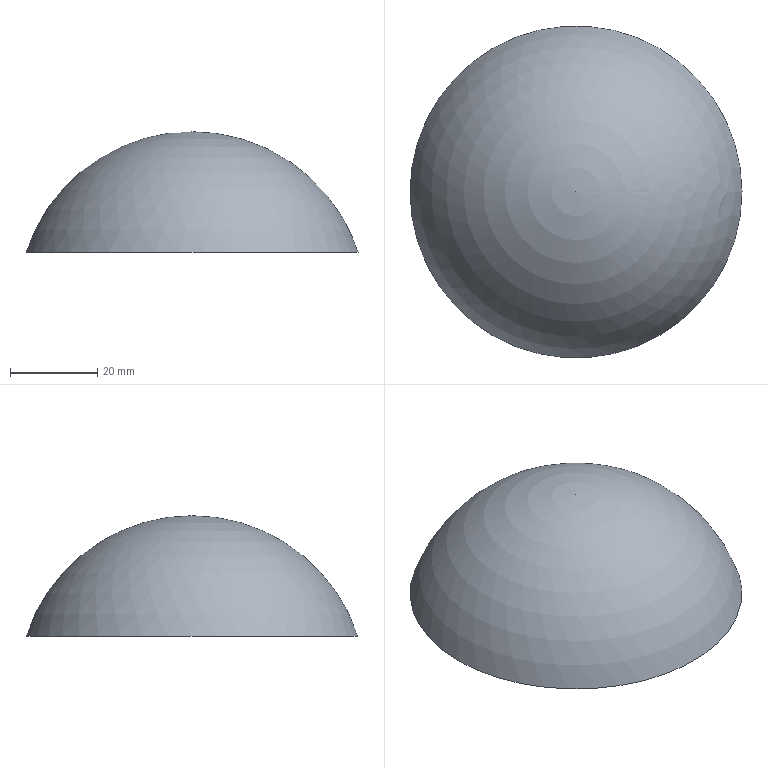Part | STEP file | 21-Guide positioning block | 1 solid | 3 faces | box 76.059 x 76.059 x 27.6 mm | volume 24483 mm3 | sphere 2 | plane 1
STEP:
#1=CARTESIAN_POINT('',(0.,0.,0.));
#2=DIRECTION('',(0.,0.,1.));
#3=DIRECTION('',(1.,0.,0.));
#4=AXIS2_PLACEMENT_3D('',#1,#2,#3);
#5=CARTESIAN_POINT('',(-38.029,0.,12.4));
#6=VERTEX_POINT('',#5);
#7=CARTESIAN_POINT('',(38.029,0.,12.4));
#8=VERTEX_POINT('',#7);
#9=CARTESIAN_POINT('',(0.,0.,12.4));
#10=DIRECTION('',(0.,0.,-1.));
#11=DIRECTION('',(-1.,0.,0.));
#12=AXIS2_PLACEMENT_3D('',#9,#10,#11);
#13=CIRCLE('',#12,38.029);
#14=CARTESIAN_POINT('',(0.,0.,0.));
#15=DIRECTION('',(0.,0.,-1.));
#16=DIRECTION('',(1.,0.,0.));
#17=AXIS2_PLACEMENT_3D('',#14,#15,#16);
#18=SPHERICAL_SURFACE('',#17,40.);
#19=CARTESIAN_POINT('',(3.142,-0.3152));
#20=DIRECTION('',(1.,0.));
#21=VECTOR('',#20,1.);
#22=LINE('',#19,#21);
#23=(GEOMETRIC_REPRESENTATION_CONTEXT(2)PARAMETRIC_REPRESENTATION_CONTEXT()REPRESENTATION_CONTEXT('',''));
#24=DEFINITIONAL_REPRESENTATION('',(#22),#23);
#25=PCURVE('',#18,#24);
#26=CARTESIAN_POINT('',(0.,0.,12.4));
#27=DIRECTION('',(0.,0.,-1.));
#28=DIRECTION('',(-1.,0.,0.));
#29=AXIS2_PLACEMENT_3D('',#26,#27,#28);
#30=PLANE('',#29);
#31=CARTESIAN_POINT('',(0.,0.));
#32=DIRECTION('',(1.,0.));
#33=AXIS2_PLACEMENT_2D('',#31,#32);
#34=CIRCLE('',#33,38.029);
#35=(GEOMETRIC_REPRESENTATION_CONTEXT(2)PARAMETRIC_REPRESENTATION_CONTEXT()REPRESENTATION_CONTEXT('',''));
#36=DEFINITIONAL_REPRESENTATION('',(#34),#35);
#37=PCURVE('',#30,#36);
#38=SURFACE_CURVE('',#13,(#25,#37),.PCURVE_S1.);
#39=EDGE_CURVE('',#6,#8,#38,.T.);
#40=ORIENTED_EDGE('',*,*,#39,.F.);
#41=CARTESIAN_POINT('',(0.,0.,12.4));
#42=DIRECTION('',(0.,0.,-1.));
#43=DIRECTION('',(-1.,0.,0.));
#44=AXIS2_PLACEMENT_3D('',#41,#42,#43);
#45=CIRCLE('',#44,38.029);
#46=CARTESIAN_POINT('',(0.,-0.3152));
#47=CARTESIAN_POINT('',(0.0476,-0.3152));
#48=CARTESIAN_POINT('',(0.1428,-0.3152));
#49=CARTESIAN_POINT('',(0.2856,-0.3152));
#50=CARTESIAN_POINT('',(0.4284,-0.3152));
#51=CARTESIAN_POINT('',(0.5712,-0.3152));
#52=CARTESIAN_POINT('',(0.714,-0.3152));
#53=CARTESIAN_POINT('',(0.8568,-0.3152));
#54=CARTESIAN_POINT('',(0.9996,-0.3152));
#55=CARTESIAN_POINT('',(1.142,-0.3152));
#56=CARTESIAN_POINT('',(1.285,-0.3152));
#57=CARTESIAN_POINT('',(1.428,-0.3152));
#58=CARTESIAN_POINT('',(1.571,-0.3152));
#59=CARTESIAN_POINT('',(1.714,-0.3152));
#60=CARTESIAN_POINT('',(1.856,-0.3152));
#61=CARTESIAN_POINT('',(1.999,-0.3152));
#62=CARTESIAN_POINT('',(2.142,-0.3152));
#63=CARTESIAN_POINT('',(2.285,-0.3152));
#64=CARTESIAN_POINT('',(2.428,-0.3152));
#65=CARTESIAN_POINT('',(2.57,-0.3152));
#66=CARTESIAN_POINT('',(2.713,-0.3152));
#67=CARTESIAN_POINT('',(2.856,-0.3152));
#68=CARTESIAN_POINT('',(2.999,-0.3152));
#69=CARTESIAN_POINT('',(3.094,-0.3152));
#70=CARTESIAN_POINT('',(3.142,-0.3152));
#71=B_SPLINE_CURVE_WITH_KNOTS('',3,(#46,#47,#48,#49,#50,#51,#52,#53,#54,#55,#56,#57,#58,#59,#60,#61,#62,#63,#64,#65,#66,#67,#68,#69,#70),.UNSPECIFIED.,.F.,.F.,(4,1,1,1,1,1,1,1,1,1,1,1,1,1,1,1,1,1,1,1,1,1,4),(3.142,3.284,3.427,3.57,3.713,3.856,3.998,4.141,4.284,4.427,4.57,4.712,4.855,4.998,5.141,5.284,5.426,5.569,5.712,5.855,5.998,6.14,6.283),.QUASI_UNIFORM_KNOTS.);
#72=(GEOMETRIC_REPRESENTATION_CONTEXT(2)PARAMETRIC_REPRESENTATION_CONTEXT()REPRESENTATION_CONTEXT('',''));
#73=DEFINITIONAL_REPRESENTATION('',(#71),#72);
#74=PCURVE('',#18,#73);
#75=CARTESIAN_POINT('',(0.,0.));
#76=DIRECTION('',(1.,0.));
#77=AXIS2_PLACEMENT_2D('',#75,#76);
#78=CIRCLE('',#77,38.029);
#79=(GEOMETRIC_REPRESENTATION_CONTEXT(2)PARAMETRIC_REPRESENTATION_CONTEXT()REPRESENTATION_CONTEXT('',''));
#80=DEFINITIONAL_REPRESENTATION('',(#78),#79);
#81=PCURVE('',#30,#80);
#82=SURFACE_CURVE('',#45,(#74,#81),.PCURVE_S1.);
#83=EDGE_CURVE('',#8,#6,#82,.T.);
#84=ORIENTED_EDGE('',*,*,#83,.F.);
#85=CARTESIAN_POINT('',(0.,0.,40.));
#86=VERTEX_POINT('',#85);
#87=CARTESIAN_POINT('',(0.,0.,40.));
#88=CARTESIAN_POINT('',(7.175,0.,40.));
#89=CARTESIAN_POINT('',(14.35,0.,38.499));
#90=CARTESIAN_POINT('',(21.148,0.,35.496));
#91=CARTESIAN_POINT('',(27.191,0.,31.109));
#92=CARTESIAN_POINT('',(32.154,0.,25.577));
#93=CARTESIAN_POINT('',(35.805,0.,19.221));
#94=CARTESIAN_POINT('',(38.029,0.,12.4));
#95=B_SPLINE_CURVE_WITH_KNOTS('',7,(#87,#88,#89,#90,#91,#92,#93,#94),.UNSPECIFIED.,.F.,.F.,(8,8),(-1.571,-0.3152),.PIECEWISE_BEZIER_KNOTS.);
#96=CARTESIAN_POINT('',(0.,0.));
#97=DIRECTION('',(0.,1.));
#98=VECTOR('',#97,1.);
#99=LINE('',#96,#98);
#100=(GEOMETRIC_REPRESENTATION_CONTEXT(2)PARAMETRIC_REPRESENTATION_CONTEXT()REPRESENTATION_CONTEXT('',''));
#101=DEFINITIONAL_REPRESENTATION('',(#99),#100);
#102=PCURVE('',#18,#101);
#103=CARTESIAN_POINT('',(6.283,0.));
#104=DIRECTION('',(0.,1.));
#105=VECTOR('',#104,1.);
#106=LINE('',#103,#105);
#107=(GEOMETRIC_REPRESENTATION_CONTEXT(2)PARAMETRIC_REPRESENTATION_CONTEXT()REPRESENTATION_CONTEXT('',''));
#108=DEFINITIONAL_REPRESENTATION('',(#106),#107);
#109=PCURVE('',#18,#108);
#110=SEAM_CURVE('',#95,(#102,#109),.PCURVE_S1.);
#111=EDGE_CURVE('',#86,#8,#110,.T.);
#112=ORIENTED_EDGE('',*,*,#111,.F.);
#113=ORIENTED_EDGE('',*,*,#111,.T.);
#114=EDGE_LOOP('',(#40,#84,#112,#113));
#115=FACE_BOUND('',#114,.T.);
#116=ADVANCED_FACE('',(#115),#18,.T.);
#117=ORIENTED_EDGE('',*,*,#39,.T.);
#118=ORIENTED_EDGE('',*,*,#83,.T.);
#119=EDGE_LOOP('',(#117,#118));
#120=FACE_BOUND('',#119,.T.);
#121=CARTESIAN_POINT('',(-33.797,0.,12.4));
#122=VERTEX_POINT('',#121);
#123=CARTESIAN_POINT('',(33.797,0.,12.4));
#124=VERTEX_POINT('',#123);
#125=CARTESIAN_POINT('',(0.,0.,12.4));
#126=DIRECTION('',(0.,0.,1.));
#127=DIRECTION('',(-1.,0.,0.));
#128=AXIS2_PLACEMENT_3D('',#125,#126,#127);
#129=CIRCLE('',#128,33.797);
#130=CARTESIAN_POINT('',(33.797,0.));
#131=CARTESIAN_POINT('',(33.797,-58.538));
#132=CARTESIAN_POINT('',(-16.899,-29.269));
#133=CARTESIAN_POINT('',(-67.594,0.));
#134=CARTESIAN_POINT('',(-16.899,29.269));
#135=CARTESIAN_POINT('',(33.797,58.538));
#136=CARTESIAN_POINT('',(33.797,0.));
#137=(BOUNDED_CURVE()B_SPLINE_CURVE(2,(#130,#131,#132,#133,#134,#135,#136),.UNSPECIFIED.,.T.,.F.)B_SPLINE_CURVE_WITH_KNOTS((1,2,2,2,2,1),(-2.094,0.,2.094,4.189,6.283,8.378),.UNSPECIFIED.)CURVE()GEOMETRIC_REPRESENTATION_ITEM()RATIONAL_B_SPLINE_CURVE((1.,0.5,1.,0.5,1.,0.5,1.))REPRESENTATION_ITEM(''));
#138=(GEOMETRIC_REPRESENTATION_CONTEXT(2)PARAMETRIC_REPRESENTATION_CONTEXT()REPRESENTATION_CONTEXT('',''));
#139=DEFINITIONAL_REPRESENTATION('',(#137),#138);
#140=PCURVE('',#30,#139);
#141=CARTESIAN_POINT('',(0.,0.,0.));
#142=DIRECTION('',(0.,0.,1.));
#143=DIRECTION('',(-1.,0.,0.));
#144=AXIS2_PLACEMENT_3D('',#141,#142,#143);
#145=SPHERICAL_SURFACE('',#144,36.);
#146=CARTESIAN_POINT('',(0.,0.3516));
#147=DIRECTION('',(1.,0.));
#148=VECTOR('',#147,1.);
#149=LINE('',#146,#148);
#150=(GEOMETRIC_REPRESENTATION_CONTEXT(2)PARAMETRIC_REPRESENTATION_CONTEXT()REPRESENTATION_CONTEXT('',''));
#151=DEFINITIONAL_REPRESENTATION('',(#149),#150);
#152=PCURVE('',#145,#151);
#153=SURFACE_CURVE('',#129,(#140,#152),.PCURVE_S1.);
#154=EDGE_CURVE('',#122,#124,#153,.T.);
#155=ORIENTED_EDGE('',*,*,#154,.T.);
#156=CARTESIAN_POINT('',(0.,0.,12.4));
#157=DIRECTION('',(0.,0.,1.));
#158=DIRECTION('',(-1.,0.,0.));
#159=AXIS2_PLACEMENT_3D('',#156,#157,#158);
#160=CIRCLE('',#159,33.797);
#161=CARTESIAN_POINT('',(33.797,0.));
#162=CARTESIAN_POINT('',(33.797,-58.538));
#163=CARTESIAN_POINT('',(-16.899,-29.269));
#164=CARTESIAN_POINT('',(-67.594,0.));
#165=CARTESIAN_POINT('',(-16.899,29.269));
#166=CARTESIAN_POINT('',(33.797,58.538));
#167=CARTESIAN_POINT('',(33.797,0.));
#168=(BOUNDED_CURVE()B_SPLINE_CURVE(2,(#161,#162,#163,#164,#165,#166,#167),.UNSPECIFIED.,.T.,.F.)B_SPLINE_CURVE_WITH_KNOTS((1,2,2,2,2,1),(-2.094,0.,2.094,4.189,6.283,8.378),.UNSPECIFIED.)CURVE()GEOMETRIC_REPRESENTATION_ITEM()RATIONAL_B_SPLINE_CURVE((1.,0.5,1.,0.5,1.,0.5,1.))REPRESENTATION_ITEM(''));
#169=(GEOMETRIC_REPRESENTATION_CONTEXT(2)PARAMETRIC_REPRESENTATION_CONTEXT()REPRESENTATION_CONTEXT('',''));
#170=DEFINITIONAL_REPRESENTATION('',(#168),#169);
#171=PCURVE('',#30,#170);
#172=CARTESIAN_POINT('',(0.,0.3516));
#173=DIRECTION('',(1.,0.));
#174=VECTOR('',#173,1.);
#175=LINE('',#172,#174);
#176=(GEOMETRIC_REPRESENTATION_CONTEXT(2)PARAMETRIC_REPRESENTATION_CONTEXT()REPRESENTATION_CONTEXT('',''));
#177=DEFINITIONAL_REPRESENTATION('',(#175),#176);
#178=PCURVE('',#145,#177);
#179=SURFACE_CURVE('',#160,(#171,#178),.PCURVE_S1.);
#180=EDGE_CURVE('',#124,#122,#179,.T.);
#181=ORIENTED_EDGE('',*,*,#180,.T.);
#182=EDGE_LOOP('',(#155,#181));
#183=FACE_BOUND('',#182,.T.);
#184=ADVANCED_FACE('',(#120,#183),#30,.T.);
#185=ORIENTED_EDGE('',*,*,#180,.T.);
#186=CARTESIAN_POINT('',(0.,0.,36.));
#187=VERTEX_POINT('',#186);
#188=CARTESIAN_POINT('',(-33.797,0.,12.4));
#189=CARTESIAN_POINT('',(-31.637,0.,18.286));
#190=CARTESIAN_POINT('',(-28.282,0.,23.734));
#191=CARTESIAN_POINT('',(-23.837,0.,28.451));
#192=CARTESIAN_POINT('',(-18.499,0.,32.178));
#193=CARTESIAN_POINT('',(-12.54,0.,34.726));
#194=CARTESIAN_POINT('',(-6.27,0.,36.));
#195=CARTESIAN_POINT('',(0.,0.,36.));
#196=B_SPLINE_CURVE_WITH_KNOTS('',7,(#188,#189,#190,#191,#192,#193,#194,#195),.UNSPECIFIED.,.F.,.F.,(8,8),(0.3516,1.571),.PIECEWISE_BEZIER_KNOTS.);
#197=CARTESIAN_POINT('',(6.283,0.));
#198=DIRECTION('',(0.,1.));
#199=VECTOR('',#198,1.);
#200=LINE('',#197,#199);
#201=(GEOMETRIC_REPRESENTATION_CONTEXT(2)PARAMETRIC_REPRESENTATION_CONTEXT()REPRESENTATION_CONTEXT('',''));
#202=DEFINITIONAL_REPRESENTATION('',(#200),#201);
#203=PCURVE('',#145,#202);
#204=CARTESIAN_POINT('',(0.,0.));
#205=DIRECTION('',(0.,1.));
#206=VECTOR('',#205,1.);
#207=LINE('',#204,#206);
#208=(GEOMETRIC_REPRESENTATION_CONTEXT(2)PARAMETRIC_REPRESENTATION_CONTEXT()REPRESENTATION_CONTEXT('',''));
#209=DEFINITIONAL_REPRESENTATION('',(#207),#208);
#210=PCURVE('',#145,#209);
#211=SEAM_CURVE('',#196,(#203,#210),.PCURVE_S1.);
#212=EDGE_CURVE('',#122,#187,#211,.T.);
#213=ORIENTED_EDGE('',*,*,#212,.T.);
#214=ORIENTED_EDGE('',*,*,#212,.F.);
#215=ORIENTED_EDGE('',*,*,#154,.T.);
#216=EDGE_LOOP('',(#185,#213,#214,#215));
#217=FACE_BOUND('',#216,.F.);
#218=ADVANCED_FACE('',(#217),#145,.F.);
#219=CLOSED_SHELL('',(#116,#184,#218));
#220=MANIFOLD_SOLID_BREP('',#219);
#221=(LENGTH_UNIT()NAMED_UNIT(*)SI_UNIT(.MILLI.,.METRE.));
#222=UNCERTAINTY_MEASURE_WITH_UNIT(LENGTH_MEASURE(0.000005),#221,'','');
#223=(NAMED_UNIT(*)PLANE_ANGLE_UNIT()SI_UNIT($,.RADIAN.));
#224=(NAMED_UNIT(*)SI_UNIT($,.STERADIAN.)SOLID_ANGLE_UNIT());
#225=(GEOMETRIC_REPRESENTATION_CONTEXT(3)GLOBAL_UNCERTAINTY_ASSIGNED_CONTEXT((#222))GLOBAL_UNIT_ASSIGNED_CONTEXT((#221,#223,#224))REPRESENTATION_CONTEXT('',''));
#226=ADVANCED_BREP_SHAPE_REPRESENTATION('',(#4,#220),#225);